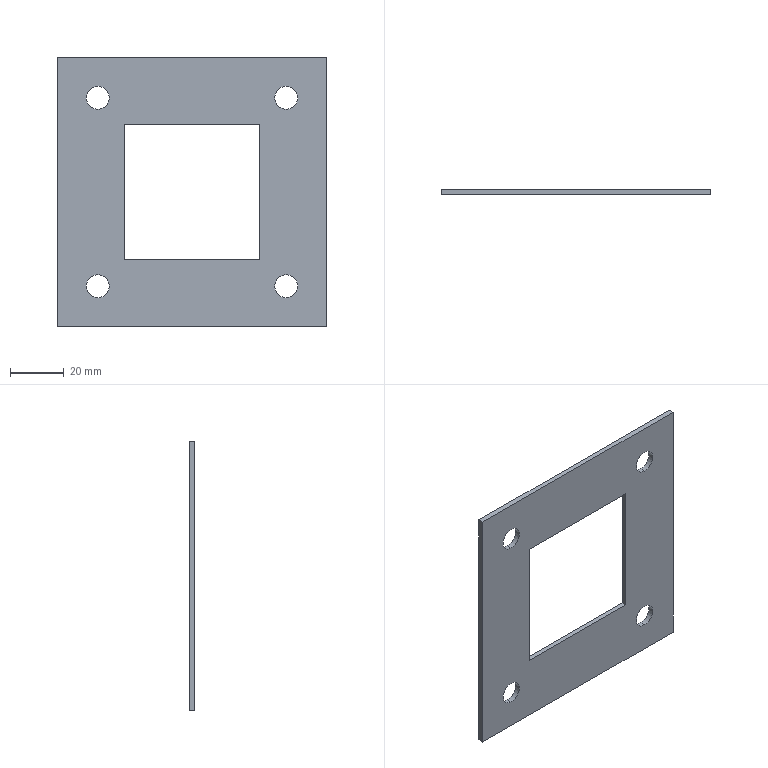Part | SolidWorks | features BaseBody 1 | 1 solid | 18 faces | box 100 x 2 x 100 mm | volume 14446 mm3 | plane 10 | cylinder 8 | commonest cylinder face diameters 8.5 x8
STEP:
#1=CARTESIAN_POINT('',(-35.,-2.,-39.25));
#2=VERTEX_POINT('',#1);
#3=CARTESIAN_POINT('',(-35.,-2.,-30.75));
#4=VERTEX_POINT('',#3);
#5=CARTESIAN_POINT('',(-35.,-2.,-35.));
#6=DIRECTION('',(0.,1.,0.));
#7=DIRECTION('',(0.,0.,1.));
#8=AXIS2_PLACEMENT_3D('',#5,#6,#7);
#9=CIRCLE('',#8,4.25);
#10=EDGE_CURVE('',#2,#4,#9,.T.);
#11=ORIENTED_EDGE('',*,*,#10,.F.);
#12=CARTESIAN_POINT('',(-35.,0.,-39.25));
#13=VERTEX_POINT('',#12);
#14=CARTESIAN_POINT('',(-35.,-10.,-39.25));
#15=DIRECTION('',(0.,1.,0.));
#16=VECTOR('',#15,1000.);
#17=LINE('',#14,#16);
#18=EDGE_CURVE('',#2,#13,#17,.T.);
#19=ORIENTED_EDGE('',*,*,#18,.T.);
#20=CARTESIAN_POINT('',(-35.,0.,-30.75));
#21=VERTEX_POINT('',#20);
#22=CARTESIAN_POINT('',(-35.,0.,-35.));
#23=DIRECTION('',(0.,-1.,0.));
#24=DIRECTION('',(0.,0.,1.));
#25=AXIS2_PLACEMENT_3D('',#22,#23,#24);
#26=CIRCLE('',#25,4.25);
#27=EDGE_CURVE('',#21,#13,#26,.T.);
#28=ORIENTED_EDGE('',*,*,#27,.F.);
#29=CARTESIAN_POINT('',(-35.,-10.,-30.75));
#30=DIRECTION('',(0.,1.,0.));
#31=VECTOR('',#30,1000.);
#32=LINE('',#29,#31);
#33=EDGE_CURVE('',#4,#21,#32,.T.);
#34=ORIENTED_EDGE('',*,*,#33,.F.);
#35=EDGE_LOOP('',(#11,#19,#28,#34));
#36=FACE_OUTER_BOUND('',#35,.T.);
#37=CARTESIAN_POINT('',(-35.,-10.,-35.));
#38=DIRECTION('',(0.,1.,0.));
#39=DIRECTION('',(0.,0.,1.));
#40=AXIS2_PLACEMENT_3D('',#37,#38,#39);
#41=CYLINDRICAL_SURFACE('',#40,4.25);
#42=ADVANCED_FACE('',(#36),#41,.F.);
#43=CARTESIAN_POINT('',(35.,-2.,-39.25));
#44=VERTEX_POINT('',#43);
#45=CARTESIAN_POINT('',(35.,-2.,-30.75));
#46=VERTEX_POINT('',#45);
#47=CARTESIAN_POINT('',(35.,-2.,-35.));
#48=DIRECTION('',(0.,1.,0.));
#49=DIRECTION('',(0.,0.,1.));
#50=AXIS2_PLACEMENT_3D('',#47,#48,#49);
#51=CIRCLE('',#50,4.25);
#52=EDGE_CURVE('',#44,#46,#51,.T.);
#53=ORIENTED_EDGE('',*,*,#52,.F.);
#54=CARTESIAN_POINT('',(35.,0.,-39.25));
#55=VERTEX_POINT('',#54);
#56=CARTESIAN_POINT('',(35.,-10.,-39.25));
#57=DIRECTION('',(0.,1.,0.));
#58=VECTOR('',#57,1000.);
#59=LINE('',#56,#58);
#60=EDGE_CURVE('',#44,#55,#59,.T.);
#61=ORIENTED_EDGE('',*,*,#60,.T.);
#62=CARTESIAN_POINT('',(35.,0.,-30.75));
#63=VERTEX_POINT('',#62);
#64=CARTESIAN_POINT('',(35.,0.,-35.));
#65=DIRECTION('',(0.,-1.,0.));
#66=DIRECTION('',(0.,0.,1.));
#67=AXIS2_PLACEMENT_3D('',#64,#65,#66);
#68=CIRCLE('',#67,4.25);
#69=EDGE_CURVE('',#63,#55,#68,.T.);
#70=ORIENTED_EDGE('',*,*,#69,.F.);
#71=CARTESIAN_POINT('',(35.,-10.,-30.75));
#72=DIRECTION('',(0.,1.,0.));
#73=VECTOR('',#72,1000.);
#74=LINE('',#71,#73);
#75=EDGE_CURVE('',#46,#63,#74,.T.);
#76=ORIENTED_EDGE('',*,*,#75,.F.);
#77=EDGE_LOOP('',(#53,#61,#70,#76));
#78=FACE_OUTER_BOUND('',#77,.T.);
#79=CARTESIAN_POINT('',(35.,-10.,-35.));
#80=DIRECTION('',(0.,1.,0.));
#81=DIRECTION('',(0.,0.,1.));
#82=AXIS2_PLACEMENT_3D('',#79,#80,#81);
#83=CYLINDRICAL_SURFACE('',#82,4.25);
#84=ADVANCED_FACE('',(#78),#83,.F.);
#85=CARTESIAN_POINT('',(35.,-2.,30.75));
#86=VERTEX_POINT('',#85);
#87=CARTESIAN_POINT('',(35.,-2.,39.25));
#88=VERTEX_POINT('',#87);
#89=CARTESIAN_POINT('',(35.,-2.,35.));
#90=DIRECTION('',(0.,1.,0.));
#91=DIRECTION('',(0.,0.,1.));
#92=AXIS2_PLACEMENT_3D('',#89,#90,#91);
#93=CIRCLE('',#92,4.25);
#94=EDGE_CURVE('',#86,#88,#93,.T.);
#95=ORIENTED_EDGE('',*,*,#94,.F.);
#96=CARTESIAN_POINT('',(35.,0.,30.75));
#97=VERTEX_POINT('',#96);
#98=CARTESIAN_POINT('',(35.,-10.,30.75));
#99=DIRECTION('',(0.,1.,0.));
#100=VECTOR('',#99,1000.);
#101=LINE('',#98,#100);
#102=EDGE_CURVE('',#86,#97,#101,.T.);
#103=ORIENTED_EDGE('',*,*,#102,.T.);
#104=CARTESIAN_POINT('',(35.,0.,39.25));
#105=VERTEX_POINT('',#104);
#106=CARTESIAN_POINT('',(35.,0.,35.));
#107=DIRECTION('',(0.,-1.,0.));
#108=DIRECTION('',(0.,0.,1.));
#109=AXIS2_PLACEMENT_3D('',#106,#107,#108);
#110=CIRCLE('',#109,4.25);
#111=EDGE_CURVE('',#105,#97,#110,.T.);
#112=ORIENTED_EDGE('',*,*,#111,.F.);
#113=CARTESIAN_POINT('',(35.,-10.,39.25));
#114=DIRECTION('',(0.,1.,0.));
#115=VECTOR('',#114,1000.);
#116=LINE('',#113,#115);
#117=EDGE_CURVE('',#88,#105,#116,.T.);
#118=ORIENTED_EDGE('',*,*,#117,.F.);
#119=EDGE_LOOP('',(#95,#103,#112,#118));
#120=FACE_OUTER_BOUND('',#119,.T.);
#121=CARTESIAN_POINT('',(35.,-10.,35.));
#122=DIRECTION('',(0.,1.,0.));
#123=DIRECTION('',(0.,0.,1.));
#124=AXIS2_PLACEMENT_3D('',#121,#122,#123);
#125=CYLINDRICAL_SURFACE('',#124,4.25);
#126=ADVANCED_FACE('',(#120),#125,.F.);
#127=CARTESIAN_POINT('',(-35.,-2.,30.75));
#128=VERTEX_POINT('',#127);
#129=CARTESIAN_POINT('',(-35.,-2.,39.25));
#130=VERTEX_POINT('',#129);
#131=CARTESIAN_POINT('',(-35.,-2.,35.));
#132=DIRECTION('',(0.,1.,0.));
#133=DIRECTION('',(0.,0.,1.));
#134=AXIS2_PLACEMENT_3D('',#131,#132,#133);
#135=CIRCLE('',#134,4.25);
#136=EDGE_CURVE('',#128,#130,#135,.T.);
#137=ORIENTED_EDGE('',*,*,#136,.F.);
#138=CARTESIAN_POINT('',(-35.,0.,30.75));
#139=VERTEX_POINT('',#138);
#140=CARTESIAN_POINT('',(-35.,-10.,30.75));
#141=DIRECTION('',(0.,1.,0.));
#142=VECTOR('',#141,1000.);
#143=LINE('',#140,#142);
#144=EDGE_CURVE('',#128,#139,#143,.T.);
#145=ORIENTED_EDGE('',*,*,#144,.T.);
#146=CARTESIAN_POINT('',(-35.,0.,39.25));
#147=VERTEX_POINT('',#146);
#148=CARTESIAN_POINT('',(-35.,0.,35.));
#149=DIRECTION('',(0.,-1.,0.));
#150=DIRECTION('',(0.,0.,1.));
#151=AXIS2_PLACEMENT_3D('',#148,#149,#150);
#152=CIRCLE('',#151,4.25);
#153=EDGE_CURVE('',#147,#139,#152,.T.);
#154=ORIENTED_EDGE('',*,*,#153,.F.);
#155=CARTESIAN_POINT('',(-35.,-10.,39.25));
#156=DIRECTION('',(0.,1.,0.));
#157=VECTOR('',#156,1000.);
#158=LINE('',#155,#157);
#159=EDGE_CURVE('',#130,#147,#158,.T.);
#160=ORIENTED_EDGE('',*,*,#159,.F.);
#161=EDGE_LOOP('',(#137,#145,#154,#160));
#162=FACE_OUTER_BOUND('',#161,.T.);
#163=CARTESIAN_POINT('',(-35.,-10.,35.));
#164=DIRECTION('',(0.,1.,0.));
#165=DIRECTION('',(0.,0.,1.));
#166=AXIS2_PLACEMENT_3D('',#163,#164,#165);
#167=CYLINDRICAL_SURFACE('',#166,4.25);
#168=ADVANCED_FACE('',(#162),#167,.F.);
#169=CARTESIAN_POINT('',(-50.,-2.,50.));
#170=VERTEX_POINT('',#169);
#171=CARTESIAN_POINT('',(-50.,-2.,-50.));
#172=VERTEX_POINT('',#171);
#173=CARTESIAN_POINT('',(-50.,-2.,0.));
#174=DIRECTION('',(0.,0.,-1.));
#175=VECTOR('',#174,1000.);
#176=LINE('',#173,#175);
#177=EDGE_CURVE('',#170,#172,#176,.T.);
#178=ORIENTED_EDGE('',*,*,#177,.T.);
#179=CARTESIAN_POINT('',(50.,-2.,-50.));
#180=VERTEX_POINT('',#179);
#181=CARTESIAN_POINT('',(0.,-2.,-50.));
#182=DIRECTION('',(1.,0.,0.));
#183=VECTOR('',#182,1000.);
#184=LINE('',#181,#183);
#185=EDGE_CURVE('',#172,#180,#184,.T.);
#186=ORIENTED_EDGE('',*,*,#185,.T.);
#187=CARTESIAN_POINT('',(50.,-2.,50.));
#188=VERTEX_POINT('',#187);
#189=CARTESIAN_POINT('',(50.,-2.,0.));
#190=DIRECTION('',(0.,0.,1.));
#191=VECTOR('',#190,1000.);
#192=LINE('',#189,#191);
#193=EDGE_CURVE('',#180,#188,#192,.T.);
#194=ORIENTED_EDGE('',*,*,#193,.T.);
#195=CARTESIAN_POINT('',(0.,-2.,50.));
#196=DIRECTION('',(-1.,0.,0.));
#197=VECTOR('',#196,1000.);
#198=LINE('',#195,#197);
#199=EDGE_CURVE('',#188,#170,#198,.T.);
#200=ORIENTED_EDGE('',*,*,#199,.T.);
#201=EDGE_LOOP('',(#178,#186,#194,#200));
#202=FACE_OUTER_BOUND('',#201,.T.);
#203=CARTESIAN_POINT('',(-25.25,-2.,-25.25));
#204=VERTEX_POINT('',#203);
#205=CARTESIAN_POINT('',(-25.25,-2.,25.25));
#206=VERTEX_POINT('',#205);
#207=CARTESIAN_POINT('',(-25.25,-2.,0.));
#208=DIRECTION('',(0.,0.,1.));
#209=VECTOR('',#208,1000.);
#210=LINE('',#207,#209);
#211=EDGE_CURVE('',#204,#206,#210,.T.);
#212=ORIENTED_EDGE('',*,*,#211,.T.);
#213=CARTESIAN_POINT('',(25.25,-2.,25.25));
#214=VERTEX_POINT('',#213);
#215=CARTESIAN_POINT('',(0.,-2.,25.25));
#216=DIRECTION('',(1.,0.,0.));
#217=VECTOR('',#216,1000.);
#218=LINE('',#215,#217);
#219=EDGE_CURVE('',#206,#214,#218,.T.);
#220=ORIENTED_EDGE('',*,*,#219,.T.);
#221=CARTESIAN_POINT('',(25.25,-2.,-25.25));
#222=VERTEX_POINT('',#221);
#223=CARTESIAN_POINT('',(25.25,-2.,0.));
#224=DIRECTION('',(0.,0.,-1.));
#225=VECTOR('',#224,1000.);
#226=LINE('',#223,#225);
#227=EDGE_CURVE('',#214,#222,#226,.T.);
#228=ORIENTED_EDGE('',*,*,#227,.T.);
#229=CARTESIAN_POINT('',(0.,-2.,-25.25));
#230=DIRECTION('',(-1.,0.,0.));
#231=VECTOR('',#230,1000.);
#232=LINE('',#229,#231);
#233=EDGE_CURVE('',#222,#204,#232,.T.);
#234=ORIENTED_EDGE('',*,*,#233,.T.);
#235=EDGE_LOOP('',(#212,#220,#228,#234));
#236=FACE_BOUND('',#235,.T.);
#237=CARTESIAN_POINT('',(-35.,-2.,-35.));
#238=DIRECTION('',(0.,1.,0.));
#239=DIRECTION('',(0.,0.,1.));
#240=AXIS2_PLACEMENT_3D('',#237,#238,#239);
#241=CIRCLE('',#240,4.25);
#242=EDGE_CURVE('',#4,#2,#241,.T.);
#243=ORIENTED_EDGE('',*,*,#242,.T.);
#244=ORIENTED_EDGE('',*,*,#10,.T.);
#245=EDGE_LOOP('',(#243,#244));
#246=FACE_BOUND('',#245,.T.);
#247=CARTESIAN_POINT('',(35.,-2.,-35.));
#248=DIRECTION('',(0.,1.,0.));
#249=DIRECTION('',(0.,0.,1.));
#250=AXIS2_PLACEMENT_3D('',#247,#248,#249);
#251=CIRCLE('',#250,4.25);
#252=EDGE_CURVE('',#46,#44,#251,.T.);
#253=ORIENTED_EDGE('',*,*,#252,.T.);
#254=ORIENTED_EDGE('',*,*,#52,.T.);
#255=EDGE_LOOP('',(#253,#254));
#256=FACE_BOUND('',#255,.T.);
#257=CARTESIAN_POINT('',(35.,-2.,35.));
#258=DIRECTION('',(0.,1.,0.));
#259=DIRECTION('',(0.,0.,1.));
#260=AXIS2_PLACEMENT_3D('',#257,#258,#259);
#261=CIRCLE('',#260,4.25);
#262=EDGE_CURVE('',#88,#86,#261,.T.);
#263=ORIENTED_EDGE('',*,*,#262,.T.);
#264=ORIENTED_EDGE('',*,*,#94,.T.);
#265=EDGE_LOOP('',(#263,#264));
#266=FACE_BOUND('',#265,.T.);
#267=CARTESIAN_POINT('',(-35.,-2.,35.));
#268=DIRECTION('',(0.,1.,0.));
#269=DIRECTION('',(0.,0.,1.));
#270=AXIS2_PLACEMENT_3D('',#267,#268,#269);
#271=CIRCLE('',#270,4.25);
#272=EDGE_CURVE('',#130,#128,#271,.T.);
#273=ORIENTED_EDGE('',*,*,#272,.T.);
#274=ORIENTED_EDGE('',*,*,#136,.T.);
#275=EDGE_LOOP('',(#273,#274));
#276=FACE_BOUND('',#275,.T.);
#277=CARTESIAN_POINT('',(0.,-2.,0.));
#278=DIRECTION('',(0.,-1.,0.));
#279=DIRECTION('',(0.,0.,-1.));
#280=AXIS2_PLACEMENT_3D('',#277,#278,#279);
#281=PLANE('',#280);
#282=ADVANCED_FACE('',(#202,#236,#246,#256,#266,#276),#281,.T.);
#283=ORIENTED_EDGE('',*,*,#185,.F.);
#284=CARTESIAN_POINT('',(-50.,0.,-50.));
#285=VERTEX_POINT('',#284);
#286=CARTESIAN_POINT('',(-50.,-2.,-50.));
#287=DIRECTION('',(0.,1.,0.));
#288=VECTOR('',#287,1000.);
#289=LINE('',#286,#288);
#290=EDGE_CURVE('',#172,#285,#289,.T.);
#291=ORIENTED_EDGE('',*,*,#290,.T.);
#292=CARTESIAN_POINT('',(50.,0.,-50.));
#293=VERTEX_POINT('',#292);
#294=CARTESIAN_POINT('',(-50.,0.,-50.));
#295=DIRECTION('',(1.,0.,0.));
#296=VECTOR('',#295,1000.);
#297=LINE('',#294,#296);
#298=EDGE_CURVE('',#285,#293,#297,.T.);
#299=ORIENTED_EDGE('',*,*,#298,.T.);
#300=CARTESIAN_POINT('',(50.,-2.,-50.));
#301=DIRECTION('',(0.,-1.,0.));
#302=VECTOR('',#301,1000.);
#303=LINE('',#300,#302);
#304=EDGE_CURVE('',#293,#180,#303,.T.);
#305=ORIENTED_EDGE('',*,*,#304,.T.);
#306=EDGE_LOOP('',(#283,#291,#299,#305));
#307=FACE_OUTER_BOUND('',#306,.T.);
#308=CARTESIAN_POINT('',(-50.,-2.,-50.));
#309=DIRECTION('',(0.,0.,-1.));
#310=DIRECTION('',(-1.,0.,0.));
#311=AXIS2_PLACEMENT_3D('',#308,#309,#310);
#312=PLANE('',#311);
#313=ADVANCED_FACE('',(#307),#312,.T.);
#314=ORIENTED_EDGE('',*,*,#177,.F.);
#315=CARTESIAN_POINT('',(-50.,0.,50.));
#316=VERTEX_POINT('',#315);
#317=CARTESIAN_POINT('',(-50.,-2.,50.));
#318=DIRECTION('',(0.,1.,0.));
#319=VECTOR('',#318,1000.);
#320=LINE('',#317,#319);
#321=EDGE_CURVE('',#170,#316,#320,.T.);
#322=ORIENTED_EDGE('',*,*,#321,.T.);
#323=CARTESIAN_POINT('',(-50.,0.,50.));
#324=DIRECTION('',(0.,0.,-1.));
#325=VECTOR('',#324,1000.);
#326=LINE('',#323,#325);
#327=EDGE_CURVE('',#316,#285,#326,.T.);
#328=ORIENTED_EDGE('',*,*,#327,.T.);
#329=ORIENTED_EDGE('',*,*,#290,.F.);
#330=EDGE_LOOP('',(#314,#322,#328,#329));
#331=FACE_OUTER_BOUND('',#330,.T.);
#332=CARTESIAN_POINT('',(-50.,-2.,50.));
#333=DIRECTION('',(-1.,0.,0.));
#334=DIRECTION('',(0.,0.,1.));
#335=AXIS2_PLACEMENT_3D('',#332,#333,#334);
#336=PLANE('',#335);
#337=ADVANCED_FACE('',(#331),#336,.T.);
#338=ORIENTED_EDGE('',*,*,#199,.F.);
#339=CARTESIAN_POINT('',(50.,0.,50.));
#340=VERTEX_POINT('',#339);
#341=CARTESIAN_POINT('',(50.,-2.,50.));
#342=DIRECTION('',(0.,1.,0.));
#343=VECTOR('',#342,1000.);
#344=LINE('',#341,#343);
#345=EDGE_CURVE('',#188,#340,#344,.T.);
#346=ORIENTED_EDGE('',*,*,#345,.T.);
#347=CARTESIAN_POINT('',(-50.,0.,50.));
#348=DIRECTION('',(-1.,0.,0.));
#349=VECTOR('',#348,1000.);
#350=LINE('',#347,#349);
#351=EDGE_CURVE('',#340,#316,#350,.T.);
#352=ORIENTED_EDGE('',*,*,#351,.T.);
#353=ORIENTED_EDGE('',*,*,#321,.F.);
#354=EDGE_LOOP('',(#338,#346,#352,#353));
#355=FACE_OUTER_BOUND('',#354,.T.);
#356=CARTESIAN_POINT('',(-50.,-2.,50.));
#357=DIRECTION('',(0.,0.,1.));
#358=DIRECTION('',(1.,0.,0.));
#359=AXIS2_PLACEMENT_3D('',#356,#357,#358);
#360=PLANE('',#359);
#361=ADVANCED_FACE('',(#355),#360,.T.);
#362=ORIENTED_EDGE('',*,*,#193,.F.);
#363=ORIENTED_EDGE('',*,*,#304,.F.);
#364=CARTESIAN_POINT('',(50.,0.,50.));
#365=DIRECTION('',(0.,0.,1.));
#366=VECTOR('',#365,1000.);
#367=LINE('',#364,#366);
#368=EDGE_CURVE('',#293,#340,#367,.T.);
#369=ORIENTED_EDGE('',*,*,#368,.T.);
#370=ORIENTED_EDGE('',*,*,#345,.F.);
#371=EDGE_LOOP('',(#362,#363,#369,#370));
#372=FACE_OUTER_BOUND('',#371,.T.);
#373=CARTESIAN_POINT('',(50.,-2.,50.));
#374=DIRECTION('',(1.,0.,0.));
#375=DIRECTION('',(0.,0.,-1.));
#376=AXIS2_PLACEMENT_3D('',#373,#374,#375);
#377=PLANE('',#376);
#378=ADVANCED_FACE('',(#372),#377,.T.);
#379=CARTESIAN_POINT('',(25.25,0.,25.25));
#380=VERTEX_POINT('',#379);
#381=CARTESIAN_POINT('',(25.25,-2.,25.25));
#382=DIRECTION('',(0.,1.,0.));
#383=VECTOR('',#382,1000.);
#384=LINE('',#381,#383);
#385=EDGE_CURVE('',#214,#380,#384,.T.);
#386=ORIENTED_EDGE('',*,*,#385,.F.);
#387=ORIENTED_EDGE('',*,*,#219,.F.);
#388=CARTESIAN_POINT('',(-25.25,0.,25.25));
#389=VERTEX_POINT('',#388);
#390=CARTESIAN_POINT('',(-25.25,-2.,25.25));
#391=DIRECTION('',(0.,-1.,0.));
#392=VECTOR('',#391,1000.);
#393=LINE('',#390,#392);
#394=EDGE_CURVE('',#389,#206,#393,.T.);
#395=ORIENTED_EDGE('',*,*,#394,.F.);
#396=CARTESIAN_POINT('',(-25.25,0.,25.25));
#397=DIRECTION('',(-1.,0.,0.));
#398=VECTOR('',#397,1000.);
#399=LINE('',#396,#398);
#400=EDGE_CURVE('',#380,#389,#399,.T.);
#401=ORIENTED_EDGE('',*,*,#400,.F.);
#402=EDGE_LOOP('',(#386,#387,#395,#401));
#403=FACE_OUTER_BOUND('',#402,.T.);
#404=CARTESIAN_POINT('',(-25.25,-2.,25.25));
#405=DIRECTION('',(0.,0.,1.));
#406=DIRECTION('',(1.,0.,0.));
#407=AXIS2_PLACEMENT_3D('',#404,#405,#406);
#408=PLANE('',#407);
#409=ADVANCED_FACE('',(#403),#408,.F.);
#410=ORIENTED_EDGE('',*,*,#394,.T.);
#411=ORIENTED_EDGE('',*,*,#211,.F.);
#412=CARTESIAN_POINT('',(-25.25,0.,-25.25));
#413=VERTEX_POINT('',#412);
#414=CARTESIAN_POINT('',(-25.25,-2.,-25.25));
#415=DIRECTION('',(0.,-1.,0.));
#416=VECTOR('',#415,1000.);
#417=LINE('',#414,#416);
#418=EDGE_CURVE('',#413,#204,#417,.T.);
#419=ORIENTED_EDGE('',*,*,#418,.F.);
#420=CARTESIAN_POINT('',(-25.25,0.,25.25));
#421=DIRECTION('',(0.,0.,-1.));
#422=VECTOR('',#421,1000.);
#423=LINE('',#420,#422);
#424=EDGE_CURVE('',#389,#413,#423,.T.);
#425=ORIENTED_EDGE('',*,*,#424,.F.);
#426=EDGE_LOOP('',(#410,#411,#419,#425));
#427=FACE_OUTER_BOUND('',#426,.T.);
#428=CARTESIAN_POINT('',(-25.25,-2.,25.25));
#429=DIRECTION('',(-1.,0.,0.));
#430=DIRECTION('',(0.,0.,1.));
#431=AXIS2_PLACEMENT_3D('',#428,#429,#430);
#432=PLANE('',#431);
#433=ADVANCED_FACE('',(#427),#432,.F.);
#434=ORIENTED_EDGE('',*,*,#418,.T.);
#435=ORIENTED_EDGE('',*,*,#233,.F.);
#436=CARTESIAN_POINT('',(25.25,0.,-25.25));
#437=VERTEX_POINT('',#436);
#438=CARTESIAN_POINT('',(25.25,-2.,-25.25));
#439=DIRECTION('',(0.,-1.,0.));
#440=VECTOR('',#439,1000.);
#441=LINE('',#438,#440);
#442=EDGE_CURVE('',#437,#222,#441,.T.);
#443=ORIENTED_EDGE('',*,*,#442,.F.);
#444=CARTESIAN_POINT('',(-25.25,0.,-25.25));
#445=DIRECTION('',(1.,0.,0.));
#446=VECTOR('',#445,1000.);
#447=LINE('',#444,#446);
#448=EDGE_CURVE('',#413,#437,#447,.T.);
#449=ORIENTED_EDGE('',*,*,#448,.F.);
#450=EDGE_LOOP('',(#434,#435,#443,#449));
#451=FACE_OUTER_BOUND('',#450,.T.);
#452=CARTESIAN_POINT('',(-25.25,-2.,-25.25));
#453=DIRECTION('',(0.,0.,-1.));
#454=DIRECTION('',(-1.,0.,0.));
#455=AXIS2_PLACEMENT_3D('',#452,#453,#454);
#456=PLANE('',#455);
#457=ADVANCED_FACE('',(#451),#456,.F.);
#458=ORIENTED_EDGE('',*,*,#442,.T.);
#459=ORIENTED_EDGE('',*,*,#227,.F.);
#460=ORIENTED_EDGE('',*,*,#385,.T.);
#461=CARTESIAN_POINT('',(25.25,0.,25.25));
#462=DIRECTION('',(0.,0.,1.));
#463=VECTOR('',#462,1000.);
#464=LINE('',#461,#463);
#465=EDGE_CURVE('',#437,#380,#464,.T.);
#466=ORIENTED_EDGE('',*,*,#465,.F.);
#467=EDGE_LOOP('',(#458,#459,#460,#466));
#468=FACE_OUTER_BOUND('',#467,.T.);
#469=CARTESIAN_POINT('',(25.25,-2.,25.25));
#470=DIRECTION('',(1.,0.,0.));
#471=DIRECTION('',(0.,0.,-1.));
#472=AXIS2_PLACEMENT_3D('',#469,#470,#471);
#473=PLANE('',#472);
#474=ADVANCED_FACE('',(#468),#473,.F.);
#475=ORIENTED_EDGE('',*,*,#18,.F.);
#476=ORIENTED_EDGE('',*,*,#242,.F.);
#477=ORIENTED_EDGE('',*,*,#33,.T.);
#478=CARTESIAN_POINT('',(-35.,0.,-35.));
#479=DIRECTION('',(0.,-1.,0.));
#480=DIRECTION('',(0.,0.,1.));
#481=AXIS2_PLACEMENT_3D('',#478,#479,#480);
#482=CIRCLE('',#481,4.25);
#483=EDGE_CURVE('',#13,#21,#482,.T.);
#484=ORIENTED_EDGE('',*,*,#483,.F.);
#485=EDGE_LOOP('',(#475,#476,#477,#484));
#486=FACE_OUTER_BOUND('',#485,.T.);
#487=CARTESIAN_POINT('',(-35.,-10.,-35.));
#488=DIRECTION('',(0.,1.,0.));
#489=DIRECTION('',(0.,0.,1.));
#490=AXIS2_PLACEMENT_3D('',#487,#488,#489);
#491=CYLINDRICAL_SURFACE('',#490,4.25);
#492=ADVANCED_FACE('',(#486),#491,.F.);
#493=ORIENTED_EDGE('',*,*,#60,.F.);
#494=ORIENTED_EDGE('',*,*,#252,.F.);
#495=ORIENTED_EDGE('',*,*,#75,.T.);
#496=CARTESIAN_POINT('',(35.,0.,-35.));
#497=DIRECTION('',(0.,-1.,0.));
#498=DIRECTION('',(0.,0.,1.));
#499=AXIS2_PLACEMENT_3D('',#496,#497,#498);
#500=CIRCLE('',#499,4.25);
#501=EDGE_CURVE('',#55,#63,#500,.T.);
#502=ORIENTED_EDGE('',*,*,#501,.F.);
#503=EDGE_LOOP('',(#493,#494,#495,#502));
#504=FACE_OUTER_BOUND('',#503,.T.);
#505=CARTESIAN_POINT('',(35.,-10.,-35.));
#506=DIRECTION('',(0.,1.,0.));
#507=DIRECTION('',(0.,0.,1.));
#508=AXIS2_PLACEMENT_3D('',#505,#506,#507);
#509=CYLINDRICAL_SURFACE('',#508,4.25);
#510=ADVANCED_FACE('',(#504),#509,.F.);
#511=ORIENTED_EDGE('',*,*,#102,.F.);
#512=ORIENTED_EDGE('',*,*,#262,.F.);
#513=ORIENTED_EDGE('',*,*,#117,.T.);
#514=CARTESIAN_POINT('',(35.,0.,35.));
#515=DIRECTION('',(0.,-1.,0.));
#516=DIRECTION('',(0.,0.,1.));
#517=AXIS2_PLACEMENT_3D('',#514,#515,#516);
#518=CIRCLE('',#517,4.25);
#519=EDGE_CURVE('',#97,#105,#518,.T.);
#520=ORIENTED_EDGE('',*,*,#519,.F.);
#521=EDGE_LOOP('',(#511,#512,#513,#520));
#522=FACE_OUTER_BOUND('',#521,.T.);
#523=CARTESIAN_POINT('',(35.,-10.,35.));
#524=DIRECTION('',(0.,1.,0.));
#525=DIRECTION('',(0.,0.,1.));
#526=AXIS2_PLACEMENT_3D('',#523,#524,#525);
#527=CYLINDRICAL_SURFACE('',#526,4.25);
#528=ADVANCED_FACE('',(#522),#527,.F.);
#529=ORIENTED_EDGE('',*,*,#144,.F.);
#530=ORIENTED_EDGE('',*,*,#272,.F.);
#531=ORIENTED_EDGE('',*,*,#159,.T.);
#532=CARTESIAN_POINT('',(-35.,0.,35.));
#533=DIRECTION('',(0.,-1.,0.));
#534=DIRECTION('',(0.,0.,1.));
#535=AXIS2_PLACEMENT_3D('',#532,#533,#534);
#536=CIRCLE('',#535,4.25);
#537=EDGE_CURVE('',#139,#147,#536,.T.);
#538=ORIENTED_EDGE('',*,*,#537,.F.);
#539=EDGE_LOOP('',(#529,#530,#531,#538));
#540=FACE_OUTER_BOUND('',#539,.T.);
#541=CARTESIAN_POINT('',(-35.,-10.,35.));
#542=DIRECTION('',(0.,1.,0.));
#543=DIRECTION('',(0.,0.,1.));
#544=AXIS2_PLACEMENT_3D('',#541,#542,#543);
#545=CYLINDRICAL_SURFACE('',#544,4.25);
#546=ADVANCED_FACE('',(#540),#545,.F.);
#547=ORIENTED_EDGE('',*,*,#298,.F.);
#548=ORIENTED_EDGE('',*,*,#327,.F.);
#549=ORIENTED_EDGE('',*,*,#351,.F.);
#550=ORIENTED_EDGE('',*,*,#368,.F.);
#551=EDGE_LOOP('',(#547,#548,#549,#550));
#552=FACE_OUTER_BOUND('',#551,.T.);
#553=ORIENTED_EDGE('',*,*,#465,.T.);
#554=ORIENTED_EDGE('',*,*,#400,.T.);
#555=ORIENTED_EDGE('',*,*,#424,.T.);
#556=ORIENTED_EDGE('',*,*,#448,.T.);
#557=EDGE_LOOP('',(#553,#554,#555,#556));
#558=FACE_BOUND('',#557,.T.);
#559=ORIENTED_EDGE('',*,*,#27,.T.);
#560=ORIENTED_EDGE('',*,*,#483,.T.);
#561=EDGE_LOOP('',(#559,#560));
#562=FACE_BOUND('',#561,.T.);
#563=ORIENTED_EDGE('',*,*,#69,.T.);
#564=ORIENTED_EDGE('',*,*,#501,.T.);
#565=EDGE_LOOP('',(#563,#564));
#566=FACE_BOUND('',#565,.T.);
#567=ORIENTED_EDGE('',*,*,#111,.T.);
#568=ORIENTED_EDGE('',*,*,#519,.T.);
#569=EDGE_LOOP('',(#567,#568));
#570=FACE_BOUND('',#569,.T.);
#571=ORIENTED_EDGE('',*,*,#153,.T.);
#572=ORIENTED_EDGE('',*,*,#537,.T.);
#573=EDGE_LOOP('',(#571,#572));
#574=FACE_BOUND('',#573,.T.);
#575=CARTESIAN_POINT('',(0.,0.,0.));
#576=DIRECTION('',(0.,-1.,0.));
#577=DIRECTION('',(0.,0.,-1.));
#578=AXIS2_PLACEMENT_3D('',#575,#576,#577);
#579=PLANE('',#578);
#580=ADVANCED_FACE('',(#552,#558,#562,#566,#570,#574),#579,.F.);
#581=CLOSED_SHELL('',(#42,#84,#126,#168,#282,#313,#337,#361,#378,#409,#433,#457,#474,#492,#510,#528,#546,#580));
#582=MANIFOLD_SOLID_BREP('',#581);
#583=CARTESIAN_POINT('',(0.,0.,0.));
#584=DIRECTION('',(0.,0.,1.));
#585=DIRECTION('',(1.,0.,0.));
#586=AXIS2_PLACEMENT_3D('',#583,#584,#585);
#587=(LENGTH_UNIT()NAMED_UNIT(*)SI_UNIT(.MILLI.,.METRE.));
#588=UNCERTAINTY_MEASURE_WITH_UNIT(LENGTH_MEASURE(0.00001),#587,'','');
#589=(NAMED_UNIT(*)PLANE_ANGLE_UNIT()SI_UNIT($,.RADIAN.));
#590=(NAMED_UNIT(*)SI_UNIT($,.STERADIAN.)SOLID_ANGLE_UNIT());
#591=(GEOMETRIC_REPRESENTATION_CONTEXT(3)GLOBAL_UNCERTAINTY_ASSIGNED_CONTEXT((#588))GLOBAL_UNIT_ASSIGNED_CONTEXT((#587,#589,#590))REPRESENTATION_CONTEXT('',''));
#592=ADVANCED_BREP_SHAPE_REPRESENTATION('',(#582,#586),#591);